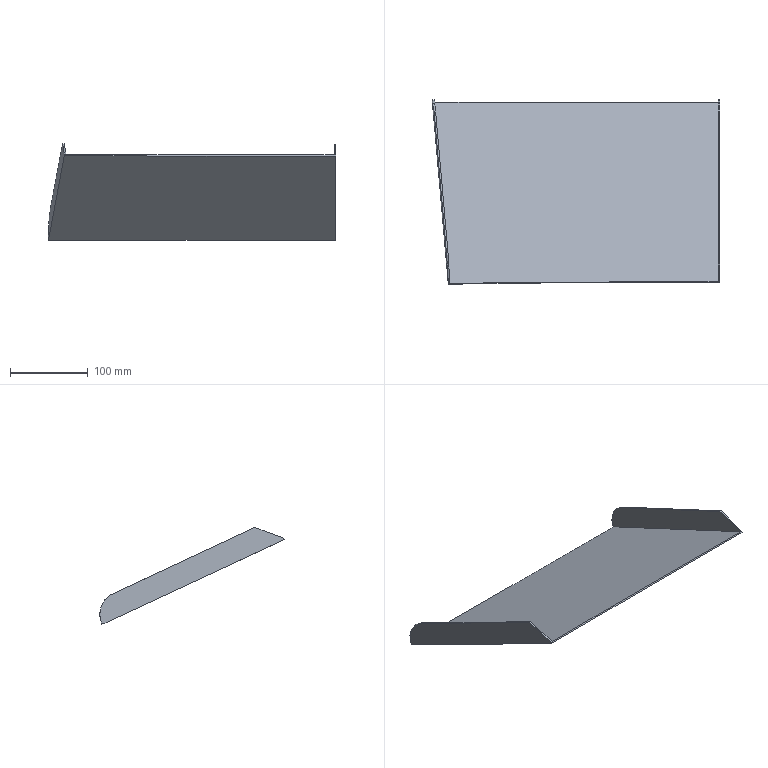Part | NX | features solid 2 | 1 solid | 14 faces | box 369.787 x 237.66 x 124.901 mm | volume 213935 mm3 | plane 11 | cylinder 2 | spline 1 | commonest cylinder face diameters 60 x2
STEP:
#1=CARTESIAN_POINT('',(775.,807.93,-206.887));
#2=VERTEX_POINT('',#1);
#3=CARTESIAN_POINT('',(425.747,805.302,-205.662));
#4=VERTEX_POINT('',#3);
#5=CARTESIAN_POINT('',(425.747,805.302,-205.662));
#6=CARTESIAN_POINT('',(429.175,805.339,-205.679));
#7=CARTESIAN_POINT('',(433.714,805.389,-205.702));
#8=CARTESIAN_POINT('',(438.558,805.443,-205.727));
#9=CARTESIAN_POINT('',(441.589,805.478,-205.744));
#10=CARTESIAN_POINT('',(444.015,805.508,-205.757));
#11=CARTESIAN_POINT('',(445.535,805.527,-205.766));
#12=CARTESIAN_POINT('',(446.449,805.54,-205.772));
#13=CARTESIAN_POINT('',(446.894,805.546,-205.775));
#14=CARTESIAN_POINT('',(447.175,805.551,-205.778));
#15=CARTESIAN_POINT('',(447.346,805.554,-205.779));
#16=CARTESIAN_POINT('',(447.466,805.557,-205.78));
#17=CARTESIAN_POINT('',(447.516,805.558,-205.781));
#18=CARTESIAN_POINT('',(447.566,805.559,-205.781));
#19=CARTESIAN_POINT('',(447.527,805.558,-205.781));
#20=CARTESIAN_POINT('',(447.771,805.565,-205.784));
#21=CARTESIAN_POINT('',(447.997,805.572,-205.787));
#22=CARTESIAN_POINT('',(448.435,805.586,-205.794));
#23=CARTESIAN_POINT('',(449.027,805.609,-205.805));
#24=CARTESIAN_POINT('',(449.733,805.642,-205.82));
#25=CARTESIAN_POINT('',(450.65,805.692,-205.843));
#26=CARTESIAN_POINT('',(451.774,805.766,-205.878));
#27=CARTESIAN_POINT('',(452.999,805.876,-205.929));
#28=CARTESIAN_POINT('',(454.167,805.974,-205.975));
#29=CARTESIAN_POINT('',(455.054,806.022,-205.997));
#30=CARTESIAN_POINT('',(455.807,806.051,-206.011));
#31=CARTESIAN_POINT('',(456.254,806.062,-206.016));
#32=CARTESIAN_POINT('',(457.117,806.081,-206.025));
#33=CARTESIAN_POINT('',(458.468,806.099,-206.033));
#34=CARTESIAN_POINT('',(460.187,806.117,-206.042));
#35=CARTESIAN_POINT('',(462.294,806.141,-206.053));
#36=CARTESIAN_POINT('',(464.717,806.169,-206.066));
#37=CARTESIAN_POINT('',(467.292,806.2,-206.08));
#38=CARTESIAN_POINT('',(470.07,806.237,-206.097));
#39=CARTESIAN_POINT('',(473.876,806.287,-206.121));
#40=CARTESIAN_POINT('',(478.642,806.347,-206.149));
#41=CARTESIAN_POINT('',(483.698,806.41,-206.178));
#42=CARTESIAN_POINT('',(489.019,806.474,-206.208));
#43=CARTESIAN_POINT('',(494.611,806.539,-206.238));
#44=CARTESIAN_POINT('',(499.496,806.594,-206.264));
#45=CARTESIAN_POINT('',(503.539,806.64,-206.285));
#46=CARTESIAN_POINT('',(506.122,806.668,-206.299));
#47=CARTESIAN_POINT('',(508.224,806.691,-206.309));
#48=CARTESIAN_POINT('',(509.813,806.709,-206.317));
#49=CARTESIAN_POINT('',(511.163,806.723,-206.324));
#50=CARTESIAN_POINT('',(512.092,806.733,-206.329));
#51=CARTESIAN_POINT('',(512.663,806.74,-206.332));
#52=CARTESIAN_POINT('',(512.983,806.743,-206.333));
#53=CARTESIAN_POINT('',(513.724,806.751,-206.337));
#54=CARTESIAN_POINT('',(514.557,806.76,-206.341));
#55=CARTESIAN_POINT('',(516.067,806.776,-206.349));
#56=CARTESIAN_POINT('',(518.14,806.799,-206.359));
#57=CARTESIAN_POINT('',(520.564,806.824,-206.371));
#58=CARTESIAN_POINT('',(523.686,806.858,-206.387));
#59=CARTESIAN_POINT('',(527.395,806.897,-206.405));
#60=CARTESIAN_POINT('',(531.532,806.94,-206.425));
#61=CARTESIAN_POINT('',(535.356,806.98,-206.444));
#62=CARTESIAN_POINT('',(540.038,807.028,-206.466));
#63=CARTESIAN_POINT('',(545.107,807.078,-206.49));
#64=CARTESIAN_POINT('',(549.133,807.116,-206.507));
#65=CARTESIAN_POINT('',(551.727,807.139,-206.518));
#66=CARTESIAN_POINT('',(553.36,807.152,-206.524));
#67=CARTESIAN_POINT('',(554.68,807.162,-206.529));
#68=CARTESIAN_POINT('',(555.519,807.167,-206.531));
#69=CARTESIAN_POINT('',(556.033,807.169,-206.532));
#70=CARTESIAN_POINT('',(556.342,807.17,-206.532));
#71=CARTESIAN_POINT('',(556.529,807.17,-206.532));
#72=CARTESIAN_POINT('',(556.637,807.169,-206.532));
#73=CARTESIAN_POINT('',(556.666,807.169,-206.532));
#74=CARTESIAN_POINT('',(556.707,807.168,-206.532));
#75=CARTESIAN_POINT('',(556.662,807.169,-206.532));
#76=CARTESIAN_POINT('',(556.899,807.165,-206.53));
#77=CARTESIAN_POINT('',(557.114,807.161,-206.528));
#78=CARTESIAN_POINT('',(557.395,807.154,-206.525));
#79=CARTESIAN_POINT('',(557.781,807.142,-206.52));
#80=CARTESIAN_POINT('',(557.932,807.136,-206.517));
#81=CARTESIAN_POINT('',(558.312,807.115,-206.507));
#82=CARTESIAN_POINT('',(558.824,807.084,-206.492));
#83=CARTESIAN_POINT('',(559.145,807.064,-206.483));
#84=CARTESIAN_POINT('',(559.476,807.044,-206.474));
#85=CARTESIAN_POINT('',(559.582,807.037,-206.471));
#86=CARTESIAN_POINT('',(559.805,807.025,-206.465));
#87=CARTESIAN_POINT('',(560.166,807.006,-206.456));
#88=CARTESIAN_POINT('',(560.73,806.98,-206.444));
#89=CARTESIAN_POINT('',(561.408,806.956,-206.433));
#90=CARTESIAN_POINT('',(562.226,806.936,-206.423));
#91=CARTESIAN_POINT('',(562.698,806.927,-206.419));
#92=CARTESIAN_POINT('',(563.51,806.916,-206.414));
#93=CARTESIAN_POINT('',(564.578,806.911,-206.412));
#94=CARTESIAN_POINT('',(565.996,806.914,-206.413));
#95=CARTESIAN_POINT('',(567.673,806.93,-206.421));
#96=CARTESIAN_POINT('',(569.065,806.947,-206.429));
#97=CARTESIAN_POINT('',(570.981,806.968,-206.438));
#98=CARTESIAN_POINT('',(573.28,806.991,-206.449));
#99=CARTESIAN_POINT('',(575.986,807.016,-206.461));
#100=CARTESIAN_POINT('',(578.493,807.035,-206.469));
#101=CARTESIAN_POINT('',(581.281,807.054,-206.478));
#102=CARTESIAN_POINT('',(584.899,807.081,-206.491));
#103=CARTESIAN_POINT('',(588.545,807.109,-206.504));
#104=CARTESIAN_POINT('',(592.182,807.138,-206.518));
#105=CARTESIAN_POINT('',(594.456,807.157,-206.527));
#106=CARTESIAN_POINT('',(596.276,807.173,-206.534));
#107=CARTESIAN_POINT('',(597.635,807.185,-206.539));
#108=CARTESIAN_POINT('',(598.789,807.195,-206.544));
#109=CARTESIAN_POINT('',(599.664,807.203,-206.548));
#110=CARTESIAN_POINT('',(600.452,807.21,-206.551));
#111=CARTESIAN_POINT('',(600.735,807.212,-206.552));
#112=CARTESIAN_POINT('',(601.302,807.217,-206.555));
#113=CARTESIAN_POINT('',(601.97,807.223,-206.557));
#114=CARTESIAN_POINT('',(602.83,807.23,-206.561));
#115=CARTESIAN_POINT('',(604.011,807.24,-206.565));
#116=CARTESIAN_POINT('',(605.57,807.252,-206.571));
#117=CARTESIAN_POINT('',(608.236,807.273,-206.58));
#118=CARTESIAN_POINT('',(611.892,807.299,-206.593));
#119=CARTESIAN_POINT('',(618.43,807.344,-206.614));
#120=CARTESIAN_POINT('',(626.001,807.392,-206.636));
#121=CARTESIAN_POINT('',(633.531,807.436,-206.657));
#122=CARTESIAN_POINT('',(638.091,807.463,-206.669));
#123=CARTESIAN_POINT('',(641.644,807.483,-206.678));
#124=CARTESIAN_POINT('',(644.7,807.5,-206.686));
#125=CARTESIAN_POINT('',(647.238,807.514,-206.693));
#126=CARTESIAN_POINT('',(648.785,807.522,-206.697));
#127=CARTESIAN_POINT('',(650.19,807.53,-206.7));
#128=CARTESIAN_POINT('',(651.051,807.535,-206.703));
#129=CARTESIAN_POINT('',(652.652,807.543,-206.707));
#130=CARTESIAN_POINT('',(655.791,807.56,-206.714));
#131=CARTESIAN_POINT('',(660.319,807.584,-206.725));
#132=CARTESIAN_POINT('',(665.756,807.611,-206.738));
#133=CARTESIAN_POINT('',(671.211,807.637,-206.75));
#134=CARTESIAN_POINT('',(676.689,807.663,-206.762));
#135=CARTESIAN_POINT('',(681.248,807.683,-206.772));
#136=CARTESIAN_POINT('',(684.947,807.699,-206.779));
#137=CARTESIAN_POINT('',(687.607,807.711,-206.785));
#138=CARTESIAN_POINT('',(690.721,807.724,-206.791));
#139=CARTESIAN_POINT('',(694.684,807.74,-206.798));
#140=CARTESIAN_POINT('',(699.647,807.76,-206.807));
#141=CARTESIAN_POINT('',(705.505,807.781,-206.818));
#142=CARTESIAN_POINT('',(713.226,807.808,-206.83));
#143=CARTESIAN_POINT('',(722.69,807.839,-206.844));
#144=CARTESIAN_POINT('',(737.44,807.879,-206.863));
#145=CARTESIAN_POINT('',(755.139,807.915,-206.88));
#146=CARTESIAN_POINT('',(768.511,807.928,-206.886));
#147=CARTESIAN_POINT('',(775.,807.93,-206.887));
#148=B_SPLINE_CURVE_WITH_KNOTS('',3,(#5,#6,#7,#8,#9,#10,#11,#12,#13,#14,#15,#16,#17,#18,#19,#20,#21,#22,#23,#24,#25,#26,#27,#28,#29,#30,#31,#32,#33,#34,#35,#36,#37,#38,#39,#40,#41,#42,#43,#44,#45,#46,#47,#48,#49,#50,#51,#52,#53,#54,#55,#56,#57,#58,#59,#60,#61,#62,#63,#64,#65,#66,#67,#68,#69,#70,#71,#72,#73,#74,#75,#76,#77,#78,#79,#80,#81,#82,#83,#84,#85,#86,#87,#88,#89,#90,#91,#92,#93,#94,#95,#96,#97,#98,#99,#100,#101,#102,#103,#104,#105,#106,#107,#108,#109,#110,#111,#112,#113,#114,#115,#116,#117,#118,#119,#120,#121,#122,#123,#124,#125,#126,#127,#128,#129,#130,#131,#132,#133,#134,#135,#136,#137,#138,#139,#140,#141,#142,#143,#144,#145,#146,#147),.UNSPECIFIED.,.F.,.F.,(4,1,1,1,1,1,1,1,1,1,1,1,1,1,1,1,1,1,1,1,1,1,1,1,1,1,1,1,1,1,1,1,1,1,1,1,1,1,1,1,1,1,1,1,1,1,1,1,1,1,1,1,1,1,1,1,1,1,1,1,1,1,1,1,1,1,1,1,1,1,1,1,1,1,1,1,1,1,1,1,1,1,1,1,1,1,1,1,1,1,1,1,1,1,1,1,1,1,1,1,1,1,1,1,1,1,1,1,1,1,1,1,1,1,1,1,1,1,1,1,1,1,1,1,1,1,1,1,1,1,1,1,1,1,1,1,1,1,1,1,4),(0.,0.01562,0.02344,0.03125,0.03906,0.04688,0.05078,0.05469,0.05664,0.05859,0.06055,0.06152,0.06201,0.0625,0.06299,0.06348,0.06445,0.06641,0.06836,0.07031,0.07422,0.07812,0.08203,0.08398,0.08594,0.08789,0.08984,0.09375,0.09766,0.1016,0.1094,0.1172,0.125,0.1406,0.1562,0.1719,0.1875,0.2031,0.2188,0.2266,0.2344,0.2383,0.2422,0.2461,0.248,0.249,0.25,0.251,0.252,0.2539,0.2578,0.2617,0.2656,0.2734,0.2812,0.2891,0.2969,0.3125,0.3281,0.3359,0.3438,0.3516,0.3594,0.3633,0.3672,0.3711,0.373,0.374,0.3745,0.375,0.3755,0.376,0.377,0.3779,0.3789,0.3809,0.3818,0.3823,0.3828,0.3833,0.3838,0.3848,0.3867,0.3887,0.3906,0.3926,0.3945,0.3984,0.4023,0.4062,0.4102,0.4141,0.4219,0.4297,0.4375,0.4453,0.4531,0.4688,0.4766,0.4844,0.4883,0.4922,0.4961,0.498,0.5,0.502,0.5039,0.5078,0.5117,0.5156,0.5234,0.5312,0.5469,0.5625,0.5938,0.6094,0.6172,0.625,0.6328,0.6367,0.6406,0.6426,0.6445,0.6484,0.6562,0.6719,0.6875,0.7031,0.7188,0.7344,0.7422,0.75,0.7578,0.7656,0.7812,0.7969,0.8125,0.8438,0.875,0.9375,1.),.UNSPECIFIED.);
#149=EDGE_CURVE('',#2,#4,#148,.F.);
#150=ORIENTED_EDGE('',*,*,#149,.F.);
#151=CARTESIAN_POINT('',(775.,808.775,-205.074));
#152=VERTEX_POINT('',#151);
#153=CARTESIAN_POINT('',(775.,808.775,-205.074));
#154=CARTESIAN_POINT('',(775.,808.493,-205.678));
#155=CARTESIAN_POINT('',(775.,808.212,-206.283));
#156=CARTESIAN_POINT('',(775.,807.93,-206.887));
#157=B_SPLINE_CURVE_WITH_KNOTS('',3,(#153,#154,#155,#156),.UNSPECIFIED.,.F.,.F.,(4,4),(0.,1.),.UNSPECIFIED.);
#158=EDGE_CURVE('',#152,#2,#157,.T.);
#159=ORIENTED_EDGE('',*,*,#158,.F.);
#160=CARTESIAN_POINT('',(773.,808.774,-205.074));
#161=VERTEX_POINT('',#160);
#162=CARTESIAN_POINT('',(773.,808.775,-205.074));
#163=CARTESIAN_POINT('',(773.667,808.775,-205.074));
#164=CARTESIAN_POINT('',(774.333,808.775,-205.074));
#165=CARTESIAN_POINT('',(775.,808.775,-205.074));
#166=B_SPLINE_CURVE_WITH_KNOTS('',3,(#162,#163,#164,#165),.UNSPECIFIED.,.F.,.F.,(4,4),(0.,1.),.UNSPECIFIED.);
#167=EDGE_CURVE('',#152,#161,#166,.F.);
#168=ORIENTED_EDGE('',*,*,#167,.T.);
#169=CARTESIAN_POINT('',(425.747,806.147,-203.849));
#170=VERTEX_POINT('',#169);
#171=CARTESIAN_POINT('',(425.747,806.147,-203.849));
#172=CARTESIAN_POINT('',(429.153,806.184,-203.866));
#173=CARTESIAN_POINT('',(433.666,806.234,-203.889));
#174=CARTESIAN_POINT('',(438.493,806.288,-203.914));
#175=CARTESIAN_POINT('',(441.517,806.323,-203.931));
#176=CARTESIAN_POINT('',(443.946,806.352,-203.944));
#177=CARTESIAN_POINT('',(445.473,806.371,-203.953));
#178=CARTESIAN_POINT('',(446.397,806.384,-203.959));
#179=CARTESIAN_POINT('',(446.85,806.391,-203.963));
#180=CARTESIAN_POINT('',(447.138,806.396,-203.965));
#181=CARTESIAN_POINT('',(447.317,806.399,-203.966));
#182=CARTESIAN_POINT('',(447.436,806.401,-203.967));
#183=CARTESIAN_POINT('',(447.51,806.403,-203.968));
#184=CARTESIAN_POINT('',(447.555,806.404,-203.969));
#185=CARTESIAN_POINT('',(447.571,806.404,-203.969));
#186=CARTESIAN_POINT('',(447.871,806.413,-203.973));
#187=CARTESIAN_POINT('',(448.261,806.426,-203.979));
#188=CARTESIAN_POINT('',(449.123,806.457,-203.994));
#189=CARTESIAN_POINT('',(450.266,806.513,-204.02));
#190=CARTESIAN_POINT('',(451.613,806.599,-204.06));
#191=CARTESIAN_POINT('',(452.848,806.705,-204.109));
#192=CARTESIAN_POINT('',(453.981,806.807,-204.156));
#193=CARTESIAN_POINT('',(454.87,806.858,-204.181));
#194=CARTESIAN_POINT('',(455.598,806.89,-204.195));
#195=CARTESIAN_POINT('',(456.111,806.904,-204.202));
#196=CARTESIAN_POINT('',(456.901,806.922,-204.21));
#197=CARTESIAN_POINT('',(458.183,806.941,-204.219));
#198=CARTESIAN_POINT('',(459.929,806.959,-204.228));
#199=CARTESIAN_POINT('',(462.034,806.983,-204.239));
#200=CARTESIAN_POINT('',(464.472,807.011,-204.252));
#201=CARTESIAN_POINT('',(467.059,807.043,-204.266));
#202=CARTESIAN_POINT('',(469.885,807.079,-204.283));
#203=CARTESIAN_POINT('',(473.594,807.129,-204.307));
#204=CARTESIAN_POINT('',(478.333,807.189,-204.335));
#205=CARTESIAN_POINT('',(483.333,807.251,-204.363));
#206=CARTESIAN_POINT('',(488.601,807.314,-204.393));
#207=CARTESIAN_POINT('',(494.136,807.379,-204.423));
#208=CARTESIAN_POINT('',(498.97,807.434,-204.449));
#209=CARTESIAN_POINT('',(502.971,807.479,-204.47));
#210=CARTESIAN_POINT('',(505.528,807.507,-204.483));
#211=CARTESIAN_POINT('',(507.606,807.53,-204.494));
#212=CARTESIAN_POINT('',(509.182,807.547,-204.502));
#213=CARTESIAN_POINT('',(510.506,807.561,-204.508));
#214=CARTESIAN_POINT('',(511.581,807.573,-204.514));
#215=CARTESIAN_POINT('',(512.241,807.58,-204.517));
#216=CARTESIAN_POINT('',(512.734,807.586,-204.52));
#217=CARTESIAN_POINT('',(512.971,807.588,-204.521));
#218=CARTESIAN_POINT('',(513.381,807.593,-204.523));
#219=CARTESIAN_POINT('',(513.93,807.598,-204.526));
#220=CARTESIAN_POINT('',(515.206,807.612,-204.532));
#221=CARTESIAN_POINT('',(517.937,807.642,-204.546));
#222=CARTESIAN_POINT('',(521.933,807.684,-204.566));
#223=CARTESIAN_POINT('',(526.425,807.732,-204.588));
#224=CARTESIAN_POINT('',(532.,807.791,-204.615));
#225=CARTESIAN_POINT('',(538.196,807.855,-204.645));
#226=CARTESIAN_POINT('',(544.396,807.917,-204.674));
#227=CARTESIAN_POINT('',(549.359,807.964,-204.696));
#228=CARTESIAN_POINT('',(552.465,807.991,-204.709));
#229=CARTESIAN_POINT('',(554.331,808.005,-204.715));
#230=CARTESIAN_POINT('',(555.422,808.012,-204.718));
#231=CARTESIAN_POINT('',(556.073,808.015,-204.72));
#232=CARTESIAN_POINT('',(556.395,808.015,-204.72));
#233=CARTESIAN_POINT('',(556.538,808.015,-204.72));
#234=CARTESIAN_POINT('',(556.617,808.014,-204.719));
#235=CARTESIAN_POINT('',(556.657,808.014,-204.719));
#236=CARTESIAN_POINT('',(556.71,808.013,-204.719));
#237=CARTESIAN_POINT('',(556.676,808.014,-204.719));
#238=CARTESIAN_POINT('',(556.977,808.009,-204.717));
#239=CARTESIAN_POINT('',(557.235,808.003,-204.714));
#240=CARTESIAN_POINT('',(557.511,807.996,-204.711));
#241=CARTESIAN_POINT('',(557.754,807.988,-204.707));
#242=CARTESIAN_POINT('',(557.863,807.984,-204.705));
#243=CARTESIAN_POINT('',(557.995,807.977,-204.702));
#244=CARTESIAN_POINT('',(558.277,807.962,-204.695));
#245=CARTESIAN_POINT('',(558.662,807.939,-204.684));
#246=CARTESIAN_POINT('',(559.031,807.917,-204.674));
#247=CARTESIAN_POINT('',(559.457,807.89,-204.662));
#248=CARTESIAN_POINT('',(559.619,807.88,-204.657));
#249=CARTESIAN_POINT('',(560.008,807.859,-204.647));
#250=CARTESIAN_POINT('',(560.538,807.834,-204.635));
#251=CARTESIAN_POINT('',(561.215,807.808,-204.623));
#252=CARTESIAN_POINT('',(561.988,807.786,-204.613));
#253=CARTESIAN_POINT('',(562.742,807.771,-204.606));
#254=CARTESIAN_POINT('',(564.102,807.755,-204.598));
#255=CARTESIAN_POINT('',(565.998,807.756,-204.599));
#256=CARTESIAN_POINT('',(568.138,807.781,-204.611));
#257=CARTESIAN_POINT('',(569.995,807.803,-204.621));
#258=CARTESIAN_POINT('',(572.344,807.827,-204.632));
#259=CARTESIAN_POINT('',(575.035,807.853,-204.644));
#260=CARTESIAN_POINT('',(577.201,807.87,-204.652));
#261=CARTESIAN_POINT('',(578.9,807.882,-204.658));
#262=CARTESIAN_POINT('',(580.734,807.895,-204.664));
#263=CARTESIAN_POINT('',(583.881,807.918,-204.675));
#264=CARTESIAN_POINT('',(587.503,807.946,-204.688));
#265=CARTESIAN_POINT('',(591.117,807.975,-204.701));
#266=CARTESIAN_POINT('',(593.827,807.997,-204.712));
#267=CARTESIAN_POINT('',(596.089,808.017,-204.721));
#268=CARTESIAN_POINT('',(597.891,808.032,-204.728));
#269=CARTESIAN_POINT('',(599.035,808.042,-204.733));
#270=CARTESIAN_POINT('',(599.8,808.049,-204.736));
#271=CARTESIAN_POINT('',(600.293,808.053,-204.738));
#272=CARTESIAN_POINT('',(600.577,808.056,-204.739));
#273=CARTESIAN_POINT('',(600.89,808.059,-204.74));
#274=CARTESIAN_POINT('',(601.427,808.063,-204.742));
#275=CARTESIAN_POINT('',(602.11,808.069,-204.745));
#276=CARTESIAN_POINT('',(603.819,808.084,-204.752));
#277=CARTESIAN_POINT('',(606.62,808.106,-204.762));
#278=CARTESIAN_POINT('',(610.866,808.137,-204.777));
#279=CARTESIAN_POINT('',(617.206,808.181,-204.797));
#280=CARTESIAN_POINT('',(624.568,808.228,-204.819));
#281=CARTESIAN_POINT('',(632.947,808.278,-204.843));
#282=CARTESIAN_POINT('',(638.614,808.311,-204.858));
#283=CARTESIAN_POINT('',(643.392,808.338,-204.87));
#284=CARTESIAN_POINT('',(646.51,808.355,-204.878));
#285=CARTESIAN_POINT('',(648.697,808.367,-204.884));
#286=CARTESIAN_POINT('',(649.874,808.373,-204.887));
#287=CARTESIAN_POINT('',(650.439,808.377,-204.888));
#288=CARTESIAN_POINT('',(650.857,808.379,-204.889));
#289=CARTESIAN_POINT('',(651.43,808.382,-204.891));
#290=CARTESIAN_POINT('',(652.32,808.387,-204.893));
#291=CARTESIAN_POINT('',(653.891,808.395,-204.897));
#292=CARTESIAN_POINT('',(656.13,808.407,-204.903));
#293=CARTESIAN_POINT('',(659.723,808.426,-204.911));
#294=CARTESIAN_POINT('',(664.222,808.449,-204.922));
#295=CARTESIAN_POINT('',(669.639,808.475,-204.934));
#296=CARTESIAN_POINT('',(675.071,808.501,-204.946));
#297=CARTESIAN_POINT('',(679.616,808.521,-204.956));
#298=CARTESIAN_POINT('',(683.249,808.537,-204.963));
#299=CARTESIAN_POINT('',(685.548,808.547,-204.968));
#300=CARTESIAN_POINT('',(687.332,808.555,-204.972));
#301=CARTESIAN_POINT('',(689.326,808.563,-204.975));
#302=CARTESIAN_POINT('',(692.817,808.578,-204.982));
#303=CARTESIAN_POINT('',(699.723,808.605,-204.995));
#304=CARTESIAN_POINT('',(709.414,808.641,-205.012));
#305=CARTESIAN_POINT('',(720.748,808.678,-205.029));
#306=CARTESIAN_POINT('',(735.472,808.72,-205.048));
#307=CARTESIAN_POINT('',(753.148,808.757,-205.066));
#308=CARTESIAN_POINT('',(766.512,808.771,-205.072));
#309=CARTESIAN_POINT('',(773.,808.774,-205.074));
#310=B_SPLINE_CURVE_WITH_KNOTS('',3,(#171,#172,#173,#174,#175,#176,#177,#178,#179,#180,#181,#182,#183,#184,#185,#186,#187,#188,#189,#190,#191,#192,#193,#194,#195,#196,#197,#198,#199,#200,#201,#202,#203,#204,#205,#206,#207,#208,#209,#210,#211,#212,#213,#214,#215,#216,#217,#218,#219,#220,#221,#222,#223,#224,#225,#226,#227,#228,#229,#230,#231,#232,#233,#234,#235,#236,#237,#238,#239,#240,#241,#242,#243,#244,#245,#246,#247,#248,#249,#250,#251,#252,#253,#254,#255,#256,#257,#258,#259,#260,#261,#262,#263,#264,#265,#266,#267,#268,#269,#270,#271,#272,#273,#274,#275,#276,#277,#278,#279,#280,#281,#282,#283,#284,#285,#286,#287,#288,#289,#290,#291,#292,#293,#294,#295,#296,#297,#298,#299,#300,#301,#302,#303,#304,#305,#306,#307,#308,#309),.UNSPECIFIED.,.F.,.F.,(4,1,1,1,1,1,1,1,1,1,1,1,1,1,1,1,1,1,1,1,1,1,1,1,1,1,1,1,1,1,1,1,1,1,1,1,1,1,1,1,1,1,1,1,1,1,1,1,1,1,1,1,1,1,1,1,1,1,1,1,1,1,1,1,1,1,1,1,1,1,1,1,1,1,1,1,1,1,1,1,1,1,1,1,1,1,1,1,1,1,1,1,1,1,1,1,1,1,1,1,1,1,1,1,1,1,1,1,1,1,1,1,1,1,1,1,1,1,1,1,1,1,1,1,1,1,1,1,1,1,1,1,1,1,1,1,4),(0.,0.01552,0.02329,0.03105,0.03881,0.04657,0.05046,0.05434,0.05628,0.05822,0.06016,0.06113,0.0621,0.06259,0.06307,0.06404,0.06598,0.06986,0.07374,0.07762,0.08151,0.08345,0.08539,0.08733,0.08927,0.09315,0.09703,0.1009,0.1087,0.1164,0.1242,0.1397,0.1552,0.1708,0.1863,0.2018,0.2173,0.2251,0.2329,0.2368,0.2406,0.2445,0.2465,0.2484,0.2494,0.2499,0.2503,0.2513,0.2523,0.2562,0.2639,0.2717,0.2794,0.295,0.3105,0.326,0.3415,0.3493,0.3571,0.3648,0.3687,0.3707,0.3726,0.3736,0.3745,0.375,0.3755,0.3765,0.3775,0.3779,0.3784,0.3794,0.3804,0.3813,0.3823,0.3828,0.3833,0.3842,0.3862,0.3881,0.3901,0.392,0.3959,0.4036,0.4075,0.4114,0.4192,0.4269,0.4347,0.4386,0.4425,0.4502,0.4657,0.4735,0.4813,0.489,0.4929,0.4968,0.4987,0.4997,0.5007,0.5026,0.5046,0.5084,0.5123,0.5278,0.5434,0.5589,0.5899,0.6055,0.621,0.6288,0.6365,0.6404,0.6423,0.6433,0.6443,0.6462,0.6482,0.652,0.6598,0.6676,0.6831,0.6986,0.7141,0.7297,0.7374,0.7452,0.7491,0.753,0.7607,0.7762,0.8073,0.8383,0.8694,0.9315,0.9936),.UNSPECIFIED.);
#311=EDGE_CURVE('',#161,#170,#310,.F.);
#312=ORIENTED_EDGE('',*,*,#311,.T.);
#313=CARTESIAN_POINT('',(425.747,805.302,-205.662));
#314=CARTESIAN_POINT('',(425.747,805.584,-205.057));
#315=CARTESIAN_POINT('',(425.747,805.866,-204.453));
#316=CARTESIAN_POINT('',(425.747,806.147,-203.849));
#317=B_SPLINE_CURVE_WITH_KNOTS('',3,(#313,#314,#315,#316),.UNSPECIFIED.,.F.,.F.,(4,4),(0.,1.),.UNSPECIFIED.);
#318=EDGE_CURVE('',#170,#4,#317,.F.);
#319=ORIENTED_EDGE('',*,*,#318,.T.);
#320=EDGE_LOOP('',(#150,#159,#168,#312,#319));
#321=FACE_BOUND('',#320,.T.);
#322=CARTESIAN_POINT('',(425.747,806.147,-203.849));
#323=CARTESIAN_POINT('',(425.747,805.302,-205.662));
#324=CARTESIAN_POINT('',(429.175,806.184,-203.866));
#325=CARTESIAN_POINT('',(429.175,805.339,-205.679));
#326=CARTESIAN_POINT('',(433.714,806.234,-203.889));
#327=CARTESIAN_POINT('',(433.714,805.389,-205.702));
#328=CARTESIAN_POINT('',(438.558,806.289,-203.915));
#329=CARTESIAN_POINT('',(438.558,805.443,-205.727));
#330=CARTESIAN_POINT('',(441.589,806.324,-203.931));
#331=CARTESIAN_POINT('',(441.589,805.478,-205.744));
#332=CARTESIAN_POINT('',(444.015,806.353,-203.945));
#333=CARTESIAN_POINT('',(444.015,805.508,-205.757));
#334=CARTESIAN_POINT('',(445.535,806.372,-203.954));
#335=CARTESIAN_POINT('',(445.535,805.527,-205.766));
#336=CARTESIAN_POINT('',(446.449,806.385,-203.96));
#337=CARTESIAN_POINT('',(446.449,805.54,-205.772));
#338=CARTESIAN_POINT('',(446.894,806.392,-203.963));
#339=CARTESIAN_POINT('',(446.894,805.546,-205.775));
#340=CARTESIAN_POINT('',(447.175,806.396,-203.965));
#341=CARTESIAN_POINT('',(447.175,805.551,-205.778));
#342=CARTESIAN_POINT('',(447.346,806.399,-203.966));
#343=CARTESIAN_POINT('',(447.346,805.554,-205.779));
#344=CARTESIAN_POINT('',(447.466,806.402,-203.968));
#345=CARTESIAN_POINT('',(447.466,805.557,-205.78));
#346=CARTESIAN_POINT('',(447.516,806.403,-203.968));
#347=CARTESIAN_POINT('',(447.516,805.558,-205.781));
#348=CARTESIAN_POINT('',(447.566,806.404,-203.969));
#349=CARTESIAN_POINT('',(447.566,805.559,-205.781));
#350=CARTESIAN_POINT('',(447.527,806.403,-203.968));
#351=CARTESIAN_POINT('',(447.527,805.558,-205.781));
#352=CARTESIAN_POINT('',(447.771,806.41,-203.971));
#353=CARTESIAN_POINT('',(447.771,805.565,-205.784));
#354=CARTESIAN_POINT('',(447.997,806.417,-203.975));
#355=CARTESIAN_POINT('',(447.997,805.572,-205.787));
#356=CARTESIAN_POINT('',(448.435,806.432,-203.981));
#357=CARTESIAN_POINT('',(448.435,805.586,-205.794));
#358=CARTESIAN_POINT('',(449.027,806.455,-203.992));
#359=CARTESIAN_POINT('',(449.027,805.609,-205.805));
#360=CARTESIAN_POINT('',(449.733,806.487,-204.007));
#361=CARTESIAN_POINT('',(449.733,805.642,-205.82));
#362=CARTESIAN_POINT('',(450.65,806.537,-204.031));
#363=CARTESIAN_POINT('',(450.65,805.692,-205.843));
#364=CARTESIAN_POINT('',(451.774,806.611,-204.065));
#365=CARTESIAN_POINT('',(451.774,805.766,-205.878));
#366=CARTESIAN_POINT('',(452.999,806.721,-204.117));
#367=CARTESIAN_POINT('',(452.999,805.876,-205.929));
#368=CARTESIAN_POINT('',(454.167,806.819,-204.162));
#369=CARTESIAN_POINT('',(454.167,805.974,-205.975));
#370=CARTESIAN_POINT('',(455.054,806.868,-204.185));
#371=CARTESIAN_POINT('',(455.054,806.022,-205.997));
#372=CARTESIAN_POINT('',(455.807,806.896,-204.198));
#373=CARTESIAN_POINT('',(455.807,806.051,-206.011));
#374=CARTESIAN_POINT('',(456.254,806.908,-204.203));
#375=CARTESIAN_POINT('',(456.254,806.062,-206.016));
#376=CARTESIAN_POINT('',(457.117,806.926,-204.212));
#377=CARTESIAN_POINT('',(457.117,806.081,-206.025));
#378=CARTESIAN_POINT('',(458.468,806.944,-204.22));
#379=CARTESIAN_POINT('',(458.468,806.099,-206.033));
#380=CARTESIAN_POINT('',(460.187,806.962,-204.229));
#381=CARTESIAN_POINT('',(460.187,806.117,-206.042));
#382=CARTESIAN_POINT('',(462.294,806.986,-204.24));
#383=CARTESIAN_POINT('',(462.294,806.141,-206.053));
#384=CARTESIAN_POINT('',(464.717,807.014,-204.253));
#385=CARTESIAN_POINT('',(464.717,806.169,-206.066));
#386=CARTESIAN_POINT('',(467.292,807.046,-204.268));
#387=CARTESIAN_POINT('',(467.292,806.2,-206.08));
#388=CARTESIAN_POINT('',(470.07,807.082,-204.285));
#389=CARTESIAN_POINT('',(470.07,806.237,-206.097));
#390=CARTESIAN_POINT('',(473.876,807.132,-204.308));
#391=CARTESIAN_POINT('',(473.876,806.287,-206.121));
#392=CARTESIAN_POINT('',(478.642,807.193,-204.336));
#393=CARTESIAN_POINT('',(478.642,806.347,-206.149));
#394=CARTESIAN_POINT('',(483.698,807.255,-204.365));
#395=CARTESIAN_POINT('',(483.698,806.41,-206.178));
#396=CARTESIAN_POINT('',(489.019,807.319,-204.395));
#397=CARTESIAN_POINT('',(489.019,806.474,-206.208));
#398=CARTESIAN_POINT('',(494.611,807.384,-204.426));
#399=CARTESIAN_POINT('',(494.611,806.539,-206.238));
#400=CARTESIAN_POINT('',(499.496,807.44,-204.452));
#401=CARTESIAN_POINT('',(499.496,806.594,-206.264));
#402=CARTESIAN_POINT('',(503.539,807.485,-204.473));
#403=CARTESIAN_POINT('',(503.539,806.64,-206.285));
#404=CARTESIAN_POINT('',(506.122,807.513,-204.486));
#405=CARTESIAN_POINT('',(506.122,806.668,-206.299));
#406=CARTESIAN_POINT('',(508.224,807.537,-204.497));
#407=CARTESIAN_POINT('',(508.224,806.691,-206.309));
#408=CARTESIAN_POINT('',(509.813,807.554,-204.505));
#409=CARTESIAN_POINT('',(509.813,806.709,-206.317));
#410=CARTESIAN_POINT('',(511.163,807.569,-204.512));
#411=CARTESIAN_POINT('',(511.163,806.723,-206.324));
#412=CARTESIAN_POINT('',(512.092,807.579,-204.516));
#413=CARTESIAN_POINT('',(512.092,806.733,-206.329));
#414=CARTESIAN_POINT('',(512.663,807.585,-204.519));
#415=CARTESIAN_POINT('',(512.663,806.74,-206.332));
#416=CARTESIAN_POINT('',(512.983,807.588,-204.521));
#417=CARTESIAN_POINT('',(512.983,806.743,-206.333));
#418=CARTESIAN_POINT('',(513.724,807.596,-204.525));
#419=CARTESIAN_POINT('',(513.724,806.751,-206.337));
#420=CARTESIAN_POINT('',(514.557,807.605,-204.529));
#421=CARTESIAN_POINT('',(514.557,806.76,-206.341));
#422=CARTESIAN_POINT('',(516.067,807.622,-204.536));
#423=CARTESIAN_POINT('',(516.067,806.776,-206.349));
#424=CARTESIAN_POINT('',(518.14,807.644,-204.547));
#425=CARTESIAN_POINT('',(518.14,806.799,-206.359));
#426=CARTESIAN_POINT('',(520.564,807.67,-204.559));
#427=CARTESIAN_POINT('',(520.564,806.824,-206.371));
#428=CARTESIAN_POINT('',(523.686,807.703,-204.574));
#429=CARTESIAN_POINT('',(523.686,806.858,-206.387));
#430=CARTESIAN_POINT('',(527.395,807.742,-204.593));
#431=CARTESIAN_POINT('',(527.395,806.897,-206.405));
#432=CARTESIAN_POINT('',(531.532,807.786,-204.613));
#433=CARTESIAN_POINT('',(531.532,806.94,-206.425));
#434=CARTESIAN_POINT('',(535.356,807.825,-204.631));
#435=CARTESIAN_POINT('',(535.356,806.98,-206.444));
#436=CARTESIAN_POINT('',(540.038,807.873,-204.654));
#437=CARTESIAN_POINT('',(540.038,807.028,-206.466));
#438=CARTESIAN_POINT('',(545.107,807.923,-204.677));
#439=CARTESIAN_POINT('',(545.107,807.078,-206.49));
#440=CARTESIAN_POINT('',(549.133,807.961,-204.695));
#441=CARTESIAN_POINT('',(549.133,807.116,-206.507));
#442=CARTESIAN_POINT('',(551.727,807.984,-204.706));
#443=CARTESIAN_POINT('',(551.727,807.139,-206.518));
#444=CARTESIAN_POINT('',(553.36,807.998,-204.712));
#445=CARTESIAN_POINT('',(553.36,807.152,-206.524));
#446=CARTESIAN_POINT('',(554.68,808.007,-204.716));
#447=CARTESIAN_POINT('',(554.68,807.162,-206.529));
#448=CARTESIAN_POINT('',(555.519,808.012,-204.719));
#449=CARTESIAN_POINT('',(555.519,807.167,-206.531));
#450=CARTESIAN_POINT('',(556.033,808.014,-204.72));
#451=CARTESIAN_POINT('',(556.033,807.169,-206.532));
#452=CARTESIAN_POINT('',(556.342,808.015,-204.72));
#453=CARTESIAN_POINT('',(556.342,807.17,-206.532));
#454=CARTESIAN_POINT('',(556.529,808.015,-204.72));
#455=CARTESIAN_POINT('',(556.529,807.17,-206.532));
#456=CARTESIAN_POINT('',(556.637,808.014,-204.719));
#457=CARTESIAN_POINT('',(556.637,807.169,-206.532));
#458=CARTESIAN_POINT('',(556.666,808.014,-204.719));
#459=CARTESIAN_POINT('',(556.666,807.169,-206.532));
#460=CARTESIAN_POINT('',(556.707,808.013,-204.719));
#461=CARTESIAN_POINT('',(556.707,807.168,-206.532));
#462=CARTESIAN_POINT('',(556.662,808.014,-204.719));
#463=CARTESIAN_POINT('',(556.662,807.169,-206.532));
#464=CARTESIAN_POINT('',(556.899,808.01,-204.718));
#465=CARTESIAN_POINT('',(556.899,807.165,-206.53));
#466=CARTESIAN_POINT('',(557.114,808.006,-204.716));
#467=CARTESIAN_POINT('',(557.114,807.161,-206.528));
#468=CARTESIAN_POINT('',(557.395,807.999,-204.713));
#469=CARTESIAN_POINT('',(557.395,807.154,-206.525));
#470=CARTESIAN_POINT('',(557.781,807.987,-204.707));
#471=CARTESIAN_POINT('',(557.781,807.142,-206.52));
#472=CARTESIAN_POINT('',(557.932,807.981,-204.704));
#473=CARTESIAN_POINT('',(557.932,807.136,-206.517));
#474=CARTESIAN_POINT('',(558.312,807.96,-204.694));
#475=CARTESIAN_POINT('',(558.312,807.115,-206.507));
#476=CARTESIAN_POINT('',(558.824,807.929,-204.68));
#477=CARTESIAN_POINT('',(558.824,807.084,-206.492));
#478=CARTESIAN_POINT('',(559.145,807.91,-204.671));
#479=CARTESIAN_POINT('',(559.145,807.064,-206.483));
#480=CARTESIAN_POINT('',(559.476,807.889,-204.661));
#481=CARTESIAN_POINT('',(559.476,807.044,-206.474));
#482=CARTESIAN_POINT('',(559.582,807.883,-204.658));
#483=CARTESIAN_POINT('',(559.582,807.037,-206.471));
#484=CARTESIAN_POINT('',(559.805,807.87,-204.652));
#485=CARTESIAN_POINT('',(559.805,807.025,-206.465));
#486=CARTESIAN_POINT('',(560.166,807.851,-204.643));
#487=CARTESIAN_POINT('',(560.166,807.006,-206.456));
#488=CARTESIAN_POINT('',(560.73,807.826,-204.631));
#489=CARTESIAN_POINT('',(560.73,806.98,-206.444));
#490=CARTESIAN_POINT('',(561.408,807.802,-204.62));
#491=CARTESIAN_POINT('',(561.408,806.956,-206.433));
#492=CARTESIAN_POINT('',(562.226,807.781,-204.611));
#493=CARTESIAN_POINT('',(562.226,806.936,-206.423));
#494=CARTESIAN_POINT('',(562.698,807.773,-204.607));
#495=CARTESIAN_POINT('',(562.698,806.927,-206.419));
#496=CARTESIAN_POINT('',(563.51,807.762,-204.602));
#497=CARTESIAN_POINT('',(563.51,806.916,-206.414));
#498=CARTESIAN_POINT('',(564.578,807.756,-204.599));
#499=CARTESIAN_POINT('',(564.578,806.911,-206.412));
#500=CARTESIAN_POINT('',(565.996,807.759,-204.6));
#501=CARTESIAN_POINT('',(565.996,806.914,-206.413));
#502=CARTESIAN_POINT('',(567.673,807.775,-204.608));
#503=CARTESIAN_POINT('',(567.673,806.93,-206.421));
#504=CARTESIAN_POINT('',(569.065,807.792,-204.616));
#505=CARTESIAN_POINT('',(569.065,806.947,-206.429));
#506=CARTESIAN_POINT('',(570.981,807.813,-204.626));
#507=CARTESIAN_POINT('',(570.981,806.968,-206.438));
#508=CARTESIAN_POINT('',(573.28,807.837,-204.637));
#509=CARTESIAN_POINT('',(573.28,806.991,-206.449));
#510=CARTESIAN_POINT('',(575.986,807.861,-204.648));
#511=CARTESIAN_POINT('',(575.986,807.016,-206.461));
#512=CARTESIAN_POINT('',(578.493,807.88,-204.657));
#513=CARTESIAN_POINT('',(578.493,807.035,-206.469));
#514=CARTESIAN_POINT('',(581.281,807.899,-204.666));
#515=CARTESIAN_POINT('',(581.281,807.054,-206.478));
#516=CARTESIAN_POINT('',(584.899,807.926,-204.678));
#517=CARTESIAN_POINT('',(584.899,807.081,-206.491));
#518=CARTESIAN_POINT('',(588.545,807.954,-204.691));
#519=CARTESIAN_POINT('',(588.545,807.109,-206.504));
#520=CARTESIAN_POINT('',(592.182,807.984,-204.705));
#521=CARTESIAN_POINT('',(592.182,807.138,-206.518));
#522=CARTESIAN_POINT('',(594.456,808.003,-204.714));
#523=CARTESIAN_POINT('',(594.456,807.157,-206.527));
#524=CARTESIAN_POINT('',(596.276,808.018,-204.721));
#525=CARTESIAN_POINT('',(596.276,807.173,-206.534));
#526=CARTESIAN_POINT('',(597.635,808.03,-204.727));
#527=CARTESIAN_POINT('',(597.635,807.185,-206.539));
#528=CARTESIAN_POINT('',(598.789,808.04,-204.732));
#529=CARTESIAN_POINT('',(598.789,807.195,-206.544));
#530=CARTESIAN_POINT('',(599.664,808.048,-204.735));
#531=CARTESIAN_POINT('',(599.664,807.203,-206.548));
#532=CARTESIAN_POINT('',(600.452,808.055,-204.738));
#533=CARTESIAN_POINT('',(600.452,807.21,-206.551));
#534=CARTESIAN_POINT('',(600.735,808.057,-204.74));
#535=CARTESIAN_POINT('',(600.735,807.212,-206.552));
#536=CARTESIAN_POINT('',(601.302,808.062,-204.742));
#537=CARTESIAN_POINT('',(601.302,807.217,-206.555));
#538=CARTESIAN_POINT('',(601.97,808.068,-204.745));
#539=CARTESIAN_POINT('',(601.97,807.223,-206.557));
#540=CARTESIAN_POINT('',(602.83,808.075,-204.748));
#541=CARTESIAN_POINT('',(602.83,807.23,-206.561));
#542=CARTESIAN_POINT('',(604.011,808.085,-204.753));
#543=CARTESIAN_POINT('',(604.011,807.24,-206.565));
#544=CARTESIAN_POINT('',(605.57,808.098,-204.758));
#545=CARTESIAN_POINT('',(605.57,807.252,-206.571));
#546=CARTESIAN_POINT('',(608.236,808.118,-204.768));
#547=CARTESIAN_POINT('',(608.236,807.273,-206.58));
#548=CARTESIAN_POINT('',(611.892,808.144,-204.78));
#549=CARTESIAN_POINT('',(611.892,807.299,-206.593));
#550=CARTESIAN_POINT('',(618.43,808.189,-204.801));
#551=CARTESIAN_POINT('',(618.43,807.344,-206.614));
#552=CARTESIAN_POINT('',(626.001,808.237,-204.823));
#553=CARTESIAN_POINT('',(626.001,807.392,-206.636));
#554=CARTESIAN_POINT('',(633.531,808.281,-204.844));
#555=CARTESIAN_POINT('',(633.531,807.436,-206.657));
#556=CARTESIAN_POINT('',(638.091,808.308,-204.856));
#557=CARTESIAN_POINT('',(638.091,807.463,-206.669));
#558=CARTESIAN_POINT('',(641.644,808.328,-204.866));
#559=CARTESIAN_POINT('',(641.644,807.483,-206.678));
#560=CARTESIAN_POINT('',(644.7,808.345,-204.874));
#561=CARTESIAN_POINT('',(644.7,807.5,-206.686));
#562=CARTESIAN_POINT('',(647.238,808.359,-204.88));
#563=CARTESIAN_POINT('',(647.238,807.514,-206.693));
#564=CARTESIAN_POINT('',(648.785,808.368,-204.884));
#565=CARTESIAN_POINT('',(648.785,807.522,-206.697));
#566=CARTESIAN_POINT('',(650.19,808.375,-204.888));
#567=CARTESIAN_POINT('',(650.19,807.53,-206.7));
#568=CARTESIAN_POINT('',(651.051,808.38,-204.89));
#569=CARTESIAN_POINT('',(651.051,807.535,-206.703));
#570=CARTESIAN_POINT('',(652.652,808.389,-204.894));
#571=CARTESIAN_POINT('',(652.652,807.543,-206.707));
#572=CARTESIAN_POINT('',(655.791,808.405,-204.902));
#573=CARTESIAN_POINT('',(655.791,807.56,-206.714));
#574=CARTESIAN_POINT('',(660.319,808.429,-204.913));
#575=CARTESIAN_POINT('',(660.319,807.584,-206.725));
#576=CARTESIAN_POINT('',(665.756,808.456,-204.926));
#577=CARTESIAN_POINT('',(665.756,807.611,-206.738));
#578=CARTESIAN_POINT('',(671.211,808.483,-204.938));
#579=CARTESIAN_POINT('',(671.211,807.637,-206.75));
#580=CARTESIAN_POINT('',(676.689,808.508,-204.95));
#581=CARTESIAN_POINT('',(676.689,807.663,-206.762));
#582=CARTESIAN_POINT('',(681.248,808.529,-204.959));
#583=CARTESIAN_POINT('',(681.248,807.683,-206.772));
#584=CARTESIAN_POINT('',(684.947,808.545,-204.967));
#585=CARTESIAN_POINT('',(684.947,807.699,-206.779));
#586=CARTESIAN_POINT('',(687.607,808.556,-204.972));
#587=CARTESIAN_POINT('',(687.607,807.711,-206.785));
#588=CARTESIAN_POINT('',(690.721,808.569,-204.978));
#589=CARTESIAN_POINT('',(690.721,807.724,-206.791));
#590=CARTESIAN_POINT('',(694.684,808.585,-204.986));
#591=CARTESIAN_POINT('',(694.684,807.74,-206.798));
#592=CARTESIAN_POINT('',(699.647,808.605,-204.995));
#593=CARTESIAN_POINT('',(699.647,807.76,-206.807));
#594=CARTESIAN_POINT('',(705.505,808.627,-205.005));
#595=CARTESIAN_POINT('',(705.505,807.781,-206.818));
#596=CARTESIAN_POINT('',(713.226,808.654,-205.018));
#597=CARTESIAN_POINT('',(713.226,807.808,-206.83));
#598=CARTESIAN_POINT('',(722.69,808.684,-205.032));
#599=CARTESIAN_POINT('',(722.69,807.839,-206.844));
#600=CARTESIAN_POINT('',(737.44,808.724,-205.051));
#601=CARTESIAN_POINT('',(737.44,807.879,-206.863));
#602=CARTESIAN_POINT('',(755.139,808.76,-205.067));
#603=CARTESIAN_POINT('',(755.139,807.915,-206.88));
#604=CARTESIAN_POINT('',(768.511,808.773,-205.073));
#605=CARTESIAN_POINT('',(768.511,807.928,-206.886));
#606=CARTESIAN_POINT('',(775.,808.775,-205.074));
#607=CARTESIAN_POINT('',(775.,807.93,-206.887));
#608=B_SPLINE_SURFACE_WITH_KNOTS('',3,1,((#322,#323),(#324,#325),(#326,#327),(#328,#329),(#330,#331),(#332,#333),(#334,#335),(#336,#337),(#338,#339),(#340,#341),(#342,#343),(#344,#345),(#346,#347),(#348,#349),(#350,#351),(#352,#353),(#354,#355),(#356,#357),(#358,#359),(#360,#361),(#362,#363),(#364,#365),(#366,#367),(#368,#369),(#370,#371),(#372,#373),(#374,#375),(#376,#377),(#378,#379),(#380,#381),(#382,#383),(#384,#385),(#386,#387),(#388,#389),(#390,#391),(#392,#393),(#394,#395),(#396,#397),(#398,#399),(#400,#401),(#402,#403),(#404,#405),(#406,#407),(#408,#409),(#410,#411),(#412,#413),(#414,#415),(#416,#417),(#418,#419),(#420,#421),(#422,#423),(#424,#425),(#426,#427),(#428,#429),(#430,#431),(#432,#433),(#434,#435),(#436,#437),(#438,#439),(#440,#441),(#442,#443),(#444,#445),(#446,#447),(#448,#449),(#450,#451),(#452,#453),(#454,#455),(#456,#457),(#458,#459),(#460,#461),(#462,#463),(#464,#465),(#466,#467),(#468,#469),(#470,#471),(#472,#473),(#474,#475),(#476,#477),(#478,#479),(#480,#481),(#482,#483),(#484,#485),(#486,#487),(#488,#489),(#490,#491),(#492,#493),(#494,#495),(#496,#497),(#498,#499),(#500,#501),(#502,#503),(#504,#505),(#506,#507),(#508,#509),(#510,#511),(#512,#513),(#514,#515),(#516,#517),(#518,#519),(#520,#521),(#522,#523),(#524,#525),(#526,#527),(#528,#529),(#530,#531),(#532,#533),(#534,#535),(#536,#537),(#538,#539),(#540,#541),(#542,#543),(#544,#545),(#546,#547),(#548,#549),(#550,#551),(#552,#553),(#554,#555),(#556,#557),(#558,#559),(#560,#561),(#562,#563),(#564,#565),(#566,#567),(#568,#569),(#570,#571),(#572,#573),(#574,#575),(#576,#577),(#578,#579),(#580,#581),(#582,#583),(#584,#585),(#586,#587),(#588,#589),(#590,#591),(#592,#593),(#594,#595),(#596,#597),(#598,#599),(#600,#601),(#602,#603),(#604,#605),(#606,#607)),.SURF_OF_LINEAR_EXTRUSION.,.F.,.F.,.F.,(4,1,1,1,1,1,1,1,1,1,1,1,1,1,1,1,1,1,1,1,1,1,1,1,1,1,1,1,1,1,1,1,1,1,1,1,1,1,1,1,1,1,1,1,1,1,1,1,1,1,1,1,1,1,1,1,1,1,1,1,1,1,1,1,1,1,1,1,1,1,1,1,1,1,1,1,1,1,1,1,1,1,1,1,1,1,1,1,1,1,1,1,1,1,1,1,1,1,1,1,1,1,1,1,1,1,1,1,1,1,1,1,1,1,1,1,1,1,1,1,1,1,1,1,1,1,1,1,1,1,1,1,1,1,1,1,1,1,1,1,4),(2,2),(0.,0.01562,0.02344,0.03125,0.03906,0.04688,0.05078,0.05469,0.05664,0.05859,0.06055,0.06152,0.06201,0.0625,0.06299,0.06348,0.06445,0.06641,0.06836,0.07031,0.07422,0.07812,0.08203,0.08398,0.08594,0.08789,0.08984,0.09375,0.09766,0.1016,0.1094,0.1172,0.125,0.1406,0.1562,0.1719,0.1875,0.2031,0.2188,0.2266,0.2344,0.2383,0.2422,0.2461,0.248,0.249,0.25,0.251,0.252,0.2539,0.2578,0.2617,0.2656,0.2734,0.2812,0.2891,0.2969,0.3125,0.3281,0.3359,0.3438,0.3516,0.3594,0.3633,0.3672,0.3711,0.373,0.374,0.3745,0.375,0.3755,0.376,0.377,0.3779,0.3789,0.3809,0.3818,0.3823,0.3828,0.3833,0.3838,0.3848,0.3867,0.3887,0.3906,0.3926,0.3945,0.3984,0.4023,0.4062,0.4102,0.4141,0.4219,0.4297,0.4375,0.4453,0.4531,0.4688,0.4766,0.4844,0.4883,0.4922,0.4961,0.498,0.5,0.502,0.5039,0.5078,0.5117,0.5156,0.5234,0.5312,0.5469,0.5625,0.5938,0.6094,0.6172,0.625,0.6328,0.6367,0.6406,0.6426,0.6445,0.6484,0.6562,0.6719,0.6875,0.7031,0.7188,0.7344,0.7422,0.75,0.7578,0.7656,0.7812,0.7969,0.8125,0.8438,0.875,0.9375,1.),(0.,1.),.UNSPECIFIED.);
#609=ADVANCED_FACE('',(#321),#608,.F.);
#610=CARTESIAN_POINT('',(775.,1040.,-315.103));
#611=VERTEX_POINT('',#610);
#612=CARTESIAN_POINT('',(775.,849.199,-226.131));
#613=DIRECTION('',(0.,-0.9063,0.4226));
#614=VECTOR('',#613,1000.);
#615=LINE('',#612,#614);
#616=EDGE_CURVE('',#611,#2,#615,.T.);
#617=ORIENTED_EDGE('',*,*,#616,.F.);
#618=CARTESIAN_POINT('',(775.,1025.489,-275.235));
#619=VERTEX_POINT('',#618);
#620=CARTESIAN_POINT('',(775.,1012.811,-302.424));
#621=DIRECTION('',(-1.,0.,0.));
#622=DIRECTION('',(0.,-1.,0.));
#623=AXIS2_PLACEMENT_3D('',#620,#621,#622);
#624=CIRCLE('',#623,30.);
#625=EDGE_CURVE('',#611,#619,#624,.F.);
#626=ORIENTED_EDGE('',*,*,#625,.T.);
#627=CARTESIAN_POINT('',(775.,845.985,-191.531));
#628=VERTEX_POINT('',#627);
#629=CARTESIAN_POINT('',(775.,1052.679,-287.914));
#630=DIRECTION('',(0.,-0.9063,0.4226));
#631=VECTOR('',#630,1000.);
#632=LINE('',#629,#631);
#633=EDGE_CURVE('',#619,#628,#632,.T.);
#634=ORIENTED_EDGE('',*,*,#633,.T.);
#635=CARTESIAN_POINT('',(775.,808.775,-205.074));
#636=DIRECTION('',(0.,-0.9397,-0.342));
#637=VECTOR('',#636,1000.);
#638=LINE('',#635,#637);
#639=EDGE_CURVE('',#628,#152,#638,.T.);
#640=ORIENTED_EDGE('',*,*,#639,.T.);
#641=ORIENTED_EDGE('',*,*,#158,.T.);
#642=EDGE_LOOP('',(#617,#626,#634,#640,#641));
#643=FACE_BOUND('',#642,.T.);
#644=CARTESIAN_POINT('',(775.,850.044,-224.318));
#645=DIRECTION('',(1.,0.,0.));
#646=DIRECTION('',(0.,0.,-1.));
#647=AXIS2_PLACEMENT_3D('',#644,#645,#646);
#648=PLANE('',#647);
#649=ADVANCED_FACE('',(#643),#648,.T.);
#650=CARTESIAN_POINT('',(407.294,1040.,-312.896));
#651=VERTEX_POINT('',#650);
#652=CARTESIAN_POINT('',(407.22,1040.,-315.103));
#653=VERTEX_POINT('',#652);
#654=CARTESIAN_POINT('',(394.59,1040.,-692.005));
#655=DIRECTION('',(0.03349,0.,0.9994));
#656=VECTOR('',#655,1000.);
#657=LINE('',#654,#656);
#658=EDGE_CURVE('',#651,#653,#657,.F.);
#659=ORIENTED_EDGE('',*,*,#658,.F.);
#660=CARTESIAN_POINT('',(773.,1040.,-312.896));
#661=VERTEX_POINT('',#660);
#662=CARTESIAN_POINT('',(885.33,1040.,-312.896));
#663=DIRECTION('',(-1.,0.,0.));
#664=VECTOR('',#663,1000.);
#665=LINE('',#662,#664);
#666=EDGE_CURVE('',#651,#661,#665,.F.);
#667=ORIENTED_EDGE('',*,*,#666,.T.);
#668=CARTESIAN_POINT('',(773.,1040.,-315.103));
#669=VERTEX_POINT('',#668);
#670=CARTESIAN_POINT('',(773.,1040.,-720.));
#671=DIRECTION('',(0.,0.,-1.));
#672=VECTOR('',#671,1000.);
#673=LINE('',#670,#672);
#674=EDGE_CURVE('',#669,#661,#673,.F.);
#675=ORIENTED_EDGE('',*,*,#674,.F.);
#676=CARTESIAN_POINT('',(885.33,1040.,-315.103));
#677=DIRECTION('',(-1.,0.,0.));
#678=VECTOR('',#677,1000.);
#679=LINE('',#676,#678);
#680=EDGE_CURVE('',#653,#669,#679,.F.);
#681=ORIENTED_EDGE('',*,*,#680,.F.);
#682=EDGE_LOOP('',(#659,#667,#675,#681));
#683=FACE_BOUND('',#682,.T.);
#684=CARTESIAN_POINT('',(1230.,1040.,-720.));
#685=DIRECTION('',(0.,-1.,0.));
#686=DIRECTION('',(-1.,0.,0.));
#687=AXIS2_PLACEMENT_3D('',#684,#685,#686);
#688=PLANE('',#687);
#689=ADVANCED_FACE('',(#683),#688,.F.);
#690=CARTESIAN_POINT('',(407.585,1025.574,-275.275));
#691=VERTEX_POINT('',#690);
#692=CARTESIAN_POINT('',(405.213,1040.,-315.103));
#693=VERTEX_POINT('',#692);
#694=CARTESIAN_POINT('',(407.585,1012.896,-302.464));
#695=DIRECTION('',(0.9969,0.07164,-0.03341));
#696=DIRECTION('',(-0.07168,0.9974,0.));
#697=AXIS2_PLACEMENT_3D('',#694,#695,#696);
#698=CIRCLE('',#697,30.);
#699=EDGE_CURVE('',#691,#693,#698,.F.);
#700=ORIENTED_EDGE('',*,*,#699,.T.);
#701=CARTESIAN_POINT('',(424.802,816.104,-210.699));
#702=DIRECTION('',(0.07904,-0.9035,0.4213));
#703=VECTOR('',#702,1000.);
#704=LINE('',#701,#703);
#705=EDGE_CURVE('',#4,#693,#704,.F.);
#706=ORIENTED_EDGE('',*,*,#705,.F.);
#707=ORIENTED_EDGE('',*,*,#318,.F.);
#708=CARTESIAN_POINT('',(423.533,843.278,-190.269));
#709=VERTEX_POINT('',#708);
#710=CARTESIAN_POINT('',(423.533,843.278,-190.269));
#711=DIRECTION('',(0.05589,-0.9377,-0.343));
#712=VECTOR('',#711,1000.);
#713=LINE('',#710,#712);
#714=EDGE_CURVE('',#170,#709,#713,.F.);
#715=ORIENTED_EDGE('',*,*,#714,.T.);
#716=CARTESIAN_POINT('',(425.747,817.981,-178.472));
#717=DIRECTION('',(-0.07904,0.9035,-0.4213));
#718=VECTOR('',#717,1000.);
#719=LINE('',#716,#718);
#720=EDGE_CURVE('',#709,#691,#719,.T.);
#721=ORIENTED_EDGE('',*,*,#720,.T.);
#722=EDGE_LOOP('',(#700,#706,#707,#715,#721));
#723=FACE_BOUND('',#722,.T.);
#724=CARTESIAN_POINT('',(424.802,816.949,-208.886));
#725=DIRECTION('',(-0.9969,-0.07164,0.03341));
#726=DIRECTION('',(0.07168,-0.9974,0.));
#727=AXIS2_PLACEMENT_3D('',#724,#725,#726);
#728=PLANE('',#727);
#729=ADVANCED_FACE('',(#723),#728,.T.);
#730=ORIENTED_EDGE('',*,*,#666,.F.);
#731=CARTESIAN_POINT('',(427.74,806.291,-203.916));
#732=VERTEX_POINT('',#731);
#733=CARTESIAN_POINT('',(426.795,817.093,-208.953));
#734=DIRECTION('',(0.07904,-0.9035,0.4213));
#735=VECTOR('',#734,1000.);
#736=LINE('',#733,#735);
#737=EDGE_CURVE('',#651,#732,#736,.T.);
#738=ORIENTED_EDGE('',*,*,#737,.T.);
#739=CARTESIAN_POINT('',(425.747,806.147,-203.849));
#740=DIRECTION('',(0.9969,0.07164,-0.03341));
#741=VECTOR('',#740,1000.);
#742=LINE('',#739,#741);
#743=EDGE_CURVE('',#732,#170,#742,.F.);
#744=ORIENTED_EDGE('',*,*,#743,.T.);
#745=ORIENTED_EDGE('',*,*,#311,.F.);
#746=CARTESIAN_POINT('',(773.,850.044,-224.318));
#747=DIRECTION('',(0.,0.9063,-0.4226));
#748=VECTOR('',#747,1000.);
#749=LINE('',#746,#748);
#750=EDGE_CURVE('',#161,#661,#749,.T.);
#751=ORIENTED_EDGE('',*,*,#750,.T.);
#752=EDGE_LOOP('',(#730,#738,#744,#745,#751));
#753=FACE_BOUND('',#752,.T.);
#754=CARTESIAN_POINT('',(885.33,850.044,-224.318));
#755=DIRECTION('',(0.,-0.4226,-0.9063));
#756=DIRECTION('',(0.,0.9063,-0.4226));
#757=AXIS2_PLACEMENT_3D('',#754,#755,#756);
#758=PLANE('',#757);
#759=ADVANCED_FACE('',(#753),#758,.F.);
#760=ORIENTED_EDGE('',*,*,#149,.T.);
#761=ORIENTED_EDGE('',*,*,#705,.T.);
#762=CARTESIAN_POINT('',(407.207,1040.143,-315.17));
#763=VERTEX_POINT('',#762);
#764=CARTESIAN_POINT('',(405.213,1040.,-315.103));
#765=DIRECTION('',(0.9969,0.07164,-0.03341));
#766=VECTOR('',#765,1000.);
#767=LINE('',#764,#766);
#768=EDGE_CURVE('',#693,#763,#767,.T.);
#769=ORIENTED_EDGE('',*,*,#768,.T.);
#770=CARTESIAN_POINT('',(427.74,805.445,-205.728));
#771=DIRECTION('',(-0.07904,0.9035,-0.4213));
#772=VECTOR('',#771,1000.);
#773=LINE('',#770,#772);
#774=EDGE_CURVE('',#653,#763,#773,.T.);
#775=ORIENTED_EDGE('',*,*,#774,.F.);
#776=ORIENTED_EDGE('',*,*,#680,.T.);
#777=CARTESIAN_POINT('',(775.,1040.,-315.103));
#778=DIRECTION('',(1.,0.,0.));
#779=VECTOR('',#778,1000.);
#780=LINE('',#777,#779);
#781=EDGE_CURVE('',#611,#669,#780,.F.);
#782=ORIENTED_EDGE('',*,*,#781,.F.);
#783=ORIENTED_EDGE('',*,*,#616,.T.);
#784=EDGE_LOOP('',(#760,#761,#769,#775,#776,#782,#783));
#785=FACE_BOUND('',#784,.T.);
#786=CARTESIAN_POINT('',(885.33,849.199,-226.131));
#787=DIRECTION('',(0.,-0.4226,-0.9063));
#788=DIRECTION('',(0.,0.9063,-0.4226));
#789=AXIS2_PLACEMENT_3D('',#786,#787,#788);
#790=PLANE('',#789);
#791=ADVANCED_FACE('',(#785),#790,.T.);
#792=CARTESIAN_POINT('',(773.,1025.489,-275.235));
#793=VERTEX_POINT('',#792);
#794=CARTESIAN_POINT('',(773.,845.985,-191.531));
#795=VERTEX_POINT('',#794);
#796=CARTESIAN_POINT('',(773.,1052.679,-287.914));
#797=DIRECTION('',(0.,-0.9063,0.4226));
#798=VECTOR('',#797,1000.);
#799=LINE('',#796,#798);
#800=EDGE_CURVE('',#793,#795,#799,.T.);
#801=ORIENTED_EDGE('',*,*,#800,.T.);
#802=CARTESIAN_POINT('',(775.,845.985,-191.531));
#803=DIRECTION('',(1.,0.,0.));
#804=VECTOR('',#803,1000.);
#805=LINE('',#802,#804);
#806=EDGE_CURVE('',#795,#628,#805,.T.);
#807=ORIENTED_EDGE('',*,*,#806,.T.);
#808=ORIENTED_EDGE('',*,*,#633,.F.);
#809=CARTESIAN_POINT('',(775.,1025.489,-275.235));
#810=DIRECTION('',(-1.,0.,0.));
#811=VECTOR('',#810,1000.);
#812=LINE('',#809,#811);
#813=EDGE_CURVE('',#619,#793,#812,.T.);
#814=ORIENTED_EDGE('',*,*,#813,.T.);
#815=EDGE_LOOP('',(#801,#807,#808,#814));
#816=FACE_BOUND('',#815,.T.);
#817=CARTESIAN_POINT('',(775.,1052.679,-287.914));
#818=DIRECTION('',(0.,-0.4226,-0.9063));
#819=DIRECTION('',(0.,-0.9063,0.4226));
#820=AXIS2_PLACEMENT_3D('',#817,#818,#819);
#821=PLANE('',#820);
#822=ADVANCED_FACE('',(#816),#821,.F.);
#823=CARTESIAN_POINT('',(773.,1012.811,-302.424));
#824=DIRECTION('',(-1.,0.,0.));
#825=DIRECTION('',(0.,-1.,0.));
#826=AXIS2_PLACEMENT_3D('',#823,#824,#825);
#827=CIRCLE('',#826,30.);
#828=EDGE_CURVE('',#793,#669,#827,.T.);
#829=ORIENTED_EDGE('',*,*,#828,.T.);
#830=ORIENTED_EDGE('',*,*,#674,.T.);
#831=ORIENTED_EDGE('',*,*,#750,.F.);
#832=CARTESIAN_POINT('',(773.,977.589,-143.631));
#833=DIRECTION('',(0.,0.9397,0.342));
#834=VECTOR('',#833,1000.);
#835=LINE('',#832,#834);
#836=EDGE_CURVE('',#161,#795,#835,.T.);
#837=ORIENTED_EDGE('',*,*,#836,.T.);
#838=ORIENTED_EDGE('',*,*,#800,.F.);
#839=EDGE_LOOP('',(#829,#830,#831,#837,#838));
#840=FACE_BOUND('',#839,.T.);
#841=CARTESIAN_POINT('',(773.,1040.,-315.103));
#842=DIRECTION('',(-1.,0.,0.));
#843=DIRECTION('',(0.,-1.,0.));
#844=AXIS2_PLACEMENT_3D('',#841,#842,#843);
#845=PLANE('',#844);
#846=ADVANCED_FACE('',(#840),#845,.T.);
#847=ORIENTED_EDGE('',*,*,#625,.F.);
#848=ORIENTED_EDGE('',*,*,#781,.T.);
#849=ORIENTED_EDGE('',*,*,#828,.F.);
#850=ORIENTED_EDGE('',*,*,#813,.F.);
#851=EDGE_LOOP('',(#847,#848,#849,#850));
#852=FACE_BOUND('',#851,.T.);
#853=CARTESIAN_POINT('',(775.,1012.811,-302.424));
#854=DIRECTION('',(-1.,0.,0.));
#855=DIRECTION('',(0.,-1.,0.));
#856=AXIS2_PLACEMENT_3D('',#853,#854,#855);
#857=CYLINDRICAL_SURFACE('',#856,30.);
#858=ADVANCED_FACE('',(#852),#857,.T.);
#859=ORIENTED_EDGE('',*,*,#639,.F.);
#860=ORIENTED_EDGE('',*,*,#806,.F.);
#861=ORIENTED_EDGE('',*,*,#836,.F.);
#862=ORIENTED_EDGE('',*,*,#167,.F.);
#863=EDGE_LOOP('',(#859,#860,#861,#862));
#864=FACE_BOUND('',#863,.T.);
#865=CARTESIAN_POINT('',(775.,808.775,-205.074));
#866=DIRECTION('',(0.,-0.342,0.9397));
#867=DIRECTION('',(0.,-0.9397,-0.342));
#868=AXIS2_PLACEMENT_3D('',#865,#866,#867);
#869=PLANE('',#868);
#870=ADVANCED_FACE('',(#864),#869,.T.);
#871=ORIENTED_EDGE('',*,*,#720,.F.);
#872=CARTESIAN_POINT('',(425.527,843.421,-190.335));
#873=VERTEX_POINT('',#872);
#874=CARTESIAN_POINT('',(423.533,843.278,-190.269));
#875=DIRECTION('',(-0.9969,-0.07164,0.03341));
#876=VECTOR('',#875,1000.);
#877=LINE('',#874,#876);
#878=EDGE_CURVE('',#709,#873,#877,.F.);
#879=ORIENTED_EDGE('',*,*,#878,.T.);
#880=CARTESIAN_POINT('',(409.578,1025.718,-275.342));
#881=VERTEX_POINT('',#880);
#882=CARTESIAN_POINT('',(427.74,818.124,-178.539));
#883=DIRECTION('',(-0.07904,0.9035,-0.4213));
#884=VECTOR('',#883,1000.);
#885=LINE('',#882,#884);
#886=EDGE_CURVE('',#873,#881,#885,.T.);
#887=ORIENTED_EDGE('',*,*,#886,.T.);
#888=CARTESIAN_POINT('',(407.585,1025.574,-275.275));
#889=DIRECTION('',(0.9969,0.07164,-0.03341));
#890=VECTOR('',#889,1000.);
#891=LINE('',#888,#890);
#892=EDGE_CURVE('',#881,#691,#891,.F.);
#893=ORIENTED_EDGE('',*,*,#892,.T.);
#894=EDGE_LOOP('',(#871,#879,#887,#893));
#895=FACE_BOUND('',#894,.T.);
#896=CARTESIAN_POINT('',(425.747,817.981,-178.472));
#897=DIRECTION('',(0.,-0.4226,-0.9063));
#898=DIRECTION('',(-0.07904,0.9035,-0.4213));
#899=AXIS2_PLACEMENT_3D('',#896,#897,#898);
#900=PLANE('',#899);
#901=ADVANCED_FACE('',(#895),#900,.F.);
#902=ORIENTED_EDGE('',*,*,#737,.F.);
#903=ORIENTED_EDGE('',*,*,#658,.T.);
#904=ORIENTED_EDGE('',*,*,#774,.T.);
#905=CARTESIAN_POINT('',(409.578,1013.039,-302.531));
#906=DIRECTION('',(0.9969,0.07164,-0.03341));
#907=DIRECTION('',(-0.07168,0.9974,0.));
#908=AXIS2_PLACEMENT_3D('',#905,#906,#907);
#909=CIRCLE('',#908,30.);
#910=EDGE_CURVE('',#763,#881,#909,.T.);
#911=ORIENTED_EDGE('',*,*,#910,.T.);
#912=ORIENTED_EDGE('',*,*,#886,.F.);
#913=CARTESIAN_POINT('',(427.819,804.965,-204.401));
#914=DIRECTION('',(-0.05589,0.9377,0.343));
#915=VECTOR('',#914,1000.);
#916=LINE('',#913,#915);
#917=EDGE_CURVE('',#873,#732,#916,.F.);
#918=ORIENTED_EDGE('',*,*,#917,.T.);
#919=EDGE_LOOP('',(#902,#903,#904,#911,#912,#918));
#920=FACE_BOUND('',#919,.T.);
#921=CARTESIAN_POINT('',(427.74,805.445,-205.728));
#922=DIRECTION('',(0.9969,0.07164,-0.03341));
#923=DIRECTION('',(-0.07168,0.9974,0.));
#924=AXIS2_PLACEMENT_3D('',#921,#922,#923);
#925=PLANE('',#924);
#926=ADVANCED_FACE('',(#920),#925,.T.);
#927=ORIENTED_EDGE('',*,*,#699,.F.);
#928=ORIENTED_EDGE('',*,*,#892,.F.);
#929=ORIENTED_EDGE('',*,*,#910,.F.);
#930=ORIENTED_EDGE('',*,*,#768,.F.);
#931=EDGE_LOOP('',(#927,#928,#929,#930));
#932=FACE_BOUND('',#931,.T.);
#933=CARTESIAN_POINT('',(407.585,1012.896,-302.464));
#934=DIRECTION('',(-0.9969,-0.07164,0.03341));
#935=DIRECTION('',(0.07168,-0.9974,0.));
#936=AXIS2_PLACEMENT_3D('',#933,#934,#935);
#937=CYLINDRICAL_SURFACE('',#936,30.);
#938=ADVANCED_FACE('',(#932),#937,.T.);
#939=ORIENTED_EDGE('',*,*,#714,.F.);
#940=ORIENTED_EDGE('',*,*,#743,.F.);
#941=ORIENTED_EDGE('',*,*,#917,.F.);
#942=ORIENTED_EDGE('',*,*,#878,.F.);
#943=EDGE_LOOP('',(#939,#940,#941,#942));
#944=FACE_BOUND('',#943,.T.);
#945=CARTESIAN_POINT('',(423.533,843.278,-190.269));
#946=DIRECTION('',(-0.05589,0.34,-0.9388));
#947=DIRECTION('',(0.,0.9402,0.3405));
#948=AXIS2_PLACEMENT_3D('',#945,#946,#947);
#949=PLANE('',#948);
#950=ADVANCED_FACE('',(#944),#949,.F.);
#951=CLOSED_SHELL('',(#609,#649,#689,#729,#759,#791,#822,#846,#858,#870,#901,#926,#938,#950));
#952=MANIFOLD_SOLID_BREP('',#951);
#953=(LENGTH_UNIT()NAMED_UNIT(*)SI_UNIT(.MILLI.,.METRE.));
#954=UNCERTAINTY_MEASURE_WITH_UNIT(LENGTH_MEASURE(0.0508),#953,'','');
#955=(NAMED_UNIT(*)PLANE_ANGLE_UNIT()SI_UNIT($,.RADIAN.));
#956=(NAMED_UNIT(*)SI_UNIT($,.STERADIAN.)SOLID_ANGLE_UNIT());
#957=(GEOMETRIC_REPRESENTATION_CONTEXT(3)GLOBAL_UNCERTAINTY_ASSIGNED_CONTEXT((#954))GLOBAL_UNIT_ASSIGNED_CONTEXT((#953,#955,#956))REPRESENTATION_CONTEXT('',''));
#958=ADVANCED_BREP_SHAPE_REPRESENTATION('',(#952),#957);